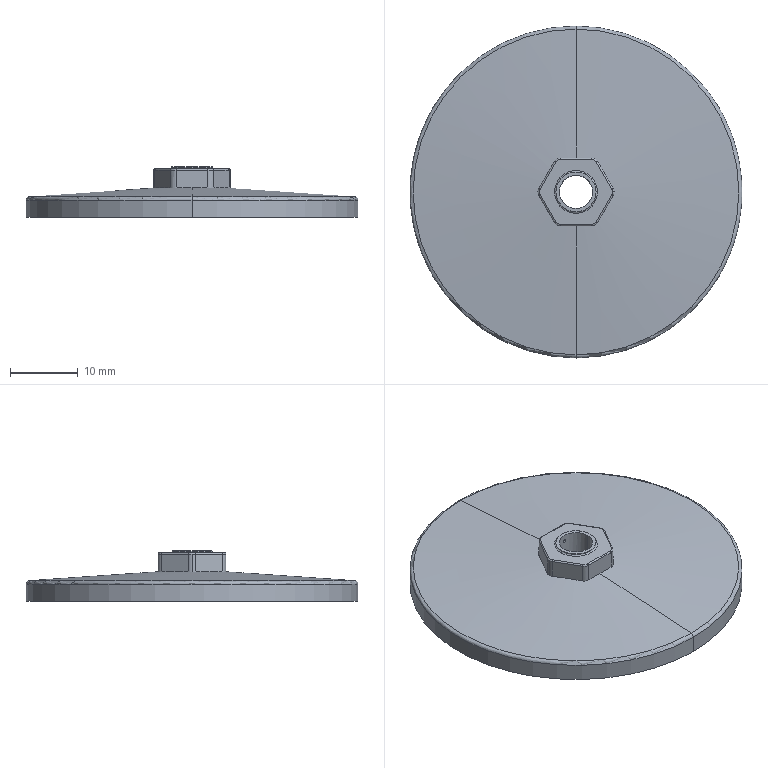Part | SolidWorks | features ICE 5, Fillet 3, BossThin 2, CirPattern 1, CutThin 1, Extrusion 1, Revolution 1 | 1 solid | 93 faces | box 49.005 x 49.005 x 7.489 mm | volume 6259 mm3 | cylinder 60 | plane 20 | torus 11 | cone 2 | commonest cylinder face diameters 46.118 x13 48.118 x13 45.836 x11 2 x7 0.4 x6 0.5 x2